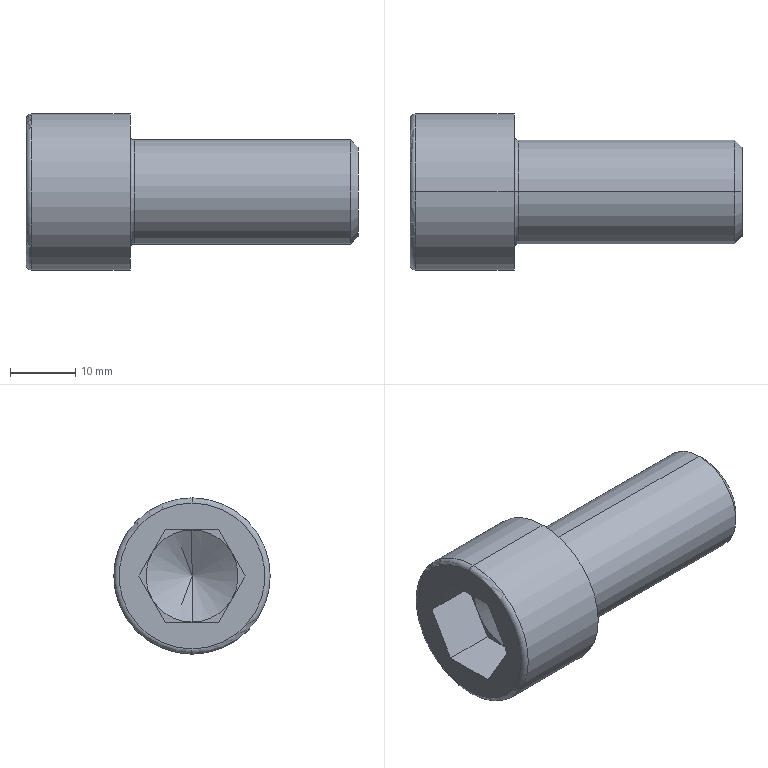Part | STEP file | socket head cap screw_iso(ISO 4762 M16 x 35 --- 35N) | 1 solid | 27 faces | box 51 x 24 x 24 mm | volume 12641 mm3 | plane 15 | cone 4 | torus 4 | cylinder 4 | commonest cylinder face diameters 16 x2 24 x2